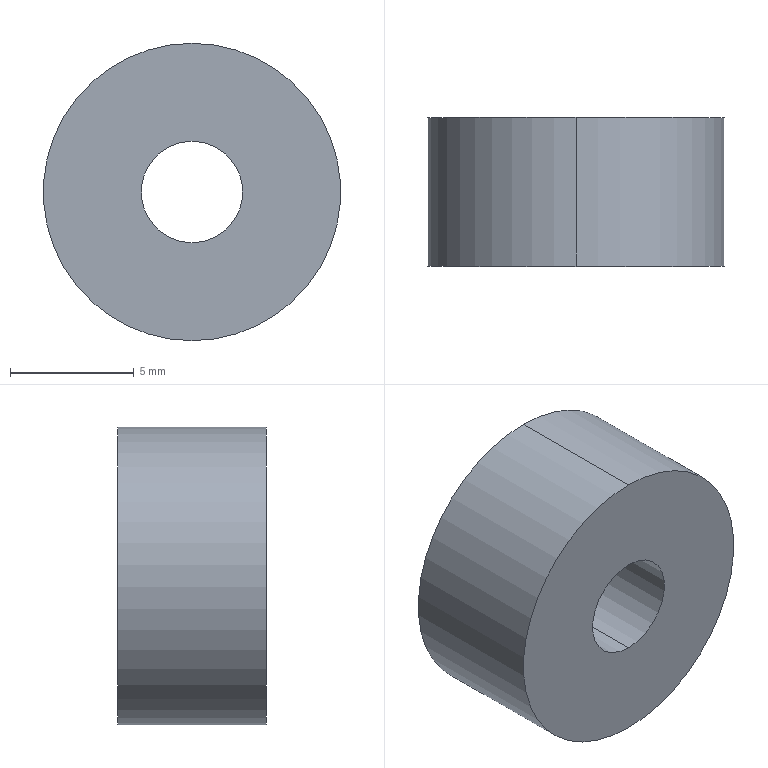Part | SolidWorks | features BaseBody 1 | 1 solid | 6 faces | box 12 x 6 x 12 mm | volume 599.369 mm3 | cylinder 4 | plane 2 | commonest cylinder face diameters 4.1 x2 12 x2
STEP:
#1=CARTESIAN_POINT('',(0.,3.,-6.));
#2=VERTEX_POINT('',#1);
#3=CARTESIAN_POINT('',(0.,3.,6.));
#4=VERTEX_POINT('',#3);
#5=CARTESIAN_POINT('',(0.,3.,0.));
#6=DIRECTION('',(0.,-1.,0.));
#7=DIRECTION('',(0.,0.,-1.));
#8=AXIS2_PLACEMENT_3D('',#5,#6,#7);
#9=CIRCLE('',#8,6.);
#10=EDGE_CURVE('',#2,#4,#9,.T.);
#11=ORIENTED_EDGE('',*,*,#10,.T.);
#12=CARTESIAN_POINT('',(0.,-3.,6.));
#13=VERTEX_POINT('',#12);
#14=CARTESIAN_POINT('',(0.,3.,6.));
#15=DIRECTION('',(0.,-1.,0.));
#16=VECTOR('',#15,1000.);
#17=LINE('',#14,#16);
#18=EDGE_CURVE('',#4,#13,#17,.T.);
#19=ORIENTED_EDGE('',*,*,#18,.T.);
#20=CARTESIAN_POINT('',(0.,-3.,-6.));
#21=VERTEX_POINT('',#20);
#22=CARTESIAN_POINT('',(0.,-3.,0.));
#23=DIRECTION('',(0.,1.,0.));
#24=DIRECTION('',(0.,0.,-1.));
#25=AXIS2_PLACEMENT_3D('',#22,#23,#24);
#26=CIRCLE('',#25,6.);
#27=EDGE_CURVE('',#13,#21,#26,.T.);
#28=ORIENTED_EDGE('',*,*,#27,.T.);
#29=CARTESIAN_POINT('',(0.,3.,-6.));
#30=DIRECTION('',(0.,-1.,0.));
#31=VECTOR('',#30,1000.);
#32=LINE('',#29,#31);
#33=EDGE_CURVE('',#2,#21,#32,.T.);
#34=ORIENTED_EDGE('',*,*,#33,.F.);
#35=EDGE_LOOP('',(#11,#19,#28,#34));
#36=FACE_OUTER_BOUND('',#35,.T.);
#37=CARTESIAN_POINT('',(0.,3.,0.));
#38=DIRECTION('',(0.,-1.,0.));
#39=DIRECTION('',(0.,0.,-1.));
#40=AXIS2_PLACEMENT_3D('',#37,#38,#39);
#41=CYLINDRICAL_SURFACE('',#40,6.);
#42=ADVANCED_FACE('',(#36),#41,.T.);
#43=CARTESIAN_POINT('',(0.,3.,2.05));
#44=VERTEX_POINT('',#43);
#45=CARTESIAN_POINT('',(0.,3.,-2.05));
#46=VERTEX_POINT('',#45);
#47=CARTESIAN_POINT('',(0.,3.,0.));
#48=DIRECTION('',(0.,-1.,0.));
#49=DIRECTION('',(0.,0.,-1.));
#50=AXIS2_PLACEMENT_3D('',#47,#48,#49);
#51=CIRCLE('',#50,2.05);
#52=EDGE_CURVE('',#44,#46,#51,.T.);
#53=ORIENTED_EDGE('',*,*,#52,.F.);
#54=CARTESIAN_POINT('',(0.,-3.,2.05));
#55=VERTEX_POINT('',#54);
#56=CARTESIAN_POINT('',(0.,3.,2.05));
#57=DIRECTION('',(0.,-1.,0.));
#58=VECTOR('',#57,1000.);
#59=LINE('',#56,#58);
#60=EDGE_CURVE('',#44,#55,#59,.T.);
#61=ORIENTED_EDGE('',*,*,#60,.T.);
#62=CARTESIAN_POINT('',(0.,-3.,-2.05));
#63=VERTEX_POINT('',#62);
#64=CARTESIAN_POINT('',(0.,-3.,0.));
#65=DIRECTION('',(0.,-1.,0.));
#66=DIRECTION('',(0.,0.,-1.));
#67=AXIS2_PLACEMENT_3D('',#64,#65,#66);
#68=CIRCLE('',#67,2.05);
#69=EDGE_CURVE('',#55,#63,#68,.T.);
#70=ORIENTED_EDGE('',*,*,#69,.T.);
#71=CARTESIAN_POINT('',(0.,3.,-2.05));
#72=DIRECTION('',(0.,-1.,0.));
#73=VECTOR('',#72,1000.);
#74=LINE('',#71,#73);
#75=EDGE_CURVE('',#46,#63,#74,.T.);
#76=ORIENTED_EDGE('',*,*,#75,.F.);
#77=EDGE_LOOP('',(#53,#61,#70,#76));
#78=FACE_OUTER_BOUND('',#77,.T.);
#79=CARTESIAN_POINT('',(0.,3.,0.));
#80=DIRECTION('',(0.,-1.,0.));
#81=DIRECTION('',(0.,0.,-1.));
#82=AXIS2_PLACEMENT_3D('',#79,#80,#81);
#83=CYLINDRICAL_SURFACE('',#82,2.05);
#84=ADVANCED_FACE('',(#78),#83,.F.);
#85=ORIENTED_EDGE('',*,*,#18,.F.);
#86=CARTESIAN_POINT('',(0.,3.,0.));
#87=DIRECTION('',(0.,-1.,0.));
#88=DIRECTION('',(0.,0.,-1.));
#89=AXIS2_PLACEMENT_3D('',#86,#87,#88);
#90=CIRCLE('',#89,6.);
#91=EDGE_CURVE('',#4,#2,#90,.T.);
#92=ORIENTED_EDGE('',*,*,#91,.T.);
#93=ORIENTED_EDGE('',*,*,#33,.T.);
#94=CARTESIAN_POINT('',(0.,-3.,0.));
#95=DIRECTION('',(0.,1.,0.));
#96=DIRECTION('',(0.,0.,-1.));
#97=AXIS2_PLACEMENT_3D('',#94,#95,#96);
#98=CIRCLE('',#97,6.);
#99=EDGE_CURVE('',#21,#13,#98,.T.);
#100=ORIENTED_EDGE('',*,*,#99,.T.);
#101=EDGE_LOOP('',(#85,#92,#93,#100));
#102=FACE_OUTER_BOUND('',#101,.T.);
#103=CARTESIAN_POINT('',(0.,3.,0.));
#104=DIRECTION('',(0.,-1.,0.));
#105=DIRECTION('',(0.,0.,-1.));
#106=AXIS2_PLACEMENT_3D('',#103,#104,#105);
#107=CYLINDRICAL_SURFACE('',#106,6.);
#108=ADVANCED_FACE('',(#102),#107,.T.);
#109=CARTESIAN_POINT('',(0.,-3.,0.));
#110=DIRECTION('',(0.,-1.,0.));
#111=DIRECTION('',(0.,0.,-1.));
#112=AXIS2_PLACEMENT_3D('',#109,#110,#111);
#113=CIRCLE('',#112,2.05);
#114=EDGE_CURVE('',#63,#55,#113,.T.);
#115=ORIENTED_EDGE('',*,*,#114,.F.);
#116=ORIENTED_EDGE('',*,*,#69,.F.);
#117=EDGE_LOOP('',(#115,#116));
#118=FACE_BOUND('',#117,.T.);
#119=ORIENTED_EDGE('',*,*,#99,.F.);
#120=ORIENTED_EDGE('',*,*,#27,.F.);
#121=EDGE_LOOP('',(#119,#120));
#122=FACE_OUTER_BOUND('',#121,.T.);
#123=CARTESIAN_POINT('',(0.,-3.,0.));
#124=DIRECTION('',(0.,1.,0.));
#125=DIRECTION('',(0.,0.,1.));
#126=AXIS2_PLACEMENT_3D('',#123,#124,#125);
#127=PLANE('',#126);
#128=ADVANCED_FACE('',(#118,#122),#127,.F.);
#129=CARTESIAN_POINT('',(0.,3.,0.));
#130=DIRECTION('',(0.,-1.,0.));
#131=DIRECTION('',(0.,0.,-1.));
#132=AXIS2_PLACEMENT_3D('',#129,#130,#131);
#133=CIRCLE('',#132,2.05);
#134=EDGE_CURVE('',#46,#44,#133,.T.);
#135=ORIENTED_EDGE('',*,*,#134,.T.);
#136=ORIENTED_EDGE('',*,*,#52,.T.);
#137=EDGE_LOOP('',(#135,#136));
#138=FACE_BOUND('',#137,.T.);
#139=ORIENTED_EDGE('',*,*,#10,.F.);
#140=ORIENTED_EDGE('',*,*,#91,.F.);
#141=EDGE_LOOP('',(#139,#140));
#142=FACE_OUTER_BOUND('',#141,.T.);
#143=CARTESIAN_POINT('',(0.,3.,0.));
#144=DIRECTION('',(0.,1.,0.));
#145=DIRECTION('',(0.,0.,1.));
#146=AXIS2_PLACEMENT_3D('',#143,#144,#145);
#147=PLANE('',#146);
#148=ADVANCED_FACE('',(#138,#142),#147,.T.);
#149=ORIENTED_EDGE('',*,*,#60,.F.);
#150=ORIENTED_EDGE('',*,*,#134,.F.);
#151=ORIENTED_EDGE('',*,*,#75,.T.);
#152=ORIENTED_EDGE('',*,*,#114,.T.);
#153=EDGE_LOOP('',(#149,#150,#151,#152));
#154=FACE_OUTER_BOUND('',#153,.T.);
#155=CARTESIAN_POINT('',(0.,3.,0.));
#156=DIRECTION('',(0.,-1.,0.));
#157=DIRECTION('',(0.,0.,-1.));
#158=AXIS2_PLACEMENT_3D('',#155,#156,#157);
#159=CYLINDRICAL_SURFACE('',#158,2.05);
#160=ADVANCED_FACE('',(#154),#159,.F.);
#161=CLOSED_SHELL('',(#42,#84,#108,#128,#148,#160));
#162=MANIFOLD_SOLID_BREP('',#161);
#163=CARTESIAN_POINT('',(0.,0.,0.));
#164=DIRECTION('',(0.,0.,1.));
#165=DIRECTION('',(1.,0.,0.));
#166=AXIS2_PLACEMENT_3D('',#163,#164,#165);
#167=(LENGTH_UNIT()NAMED_UNIT(*)SI_UNIT(.MILLI.,.METRE.));
#168=UNCERTAINTY_MEASURE_WITH_UNIT(LENGTH_MEASURE(0.00001),#167,'','');
#169=(NAMED_UNIT(*)PLANE_ANGLE_UNIT()SI_UNIT($,.RADIAN.));
#170=(NAMED_UNIT(*)SI_UNIT($,.STERADIAN.)SOLID_ANGLE_UNIT());
#171=(GEOMETRIC_REPRESENTATION_CONTEXT(3)GLOBAL_UNCERTAINTY_ASSIGNED_CONTEXT((#168))GLOBAL_UNIT_ASSIGNED_CONTEXT((#167,#169,#170))REPRESENTATION_CONTEXT('',''));
#172=ADVANCED_BREP_SHAPE_REPRESENTATION('',(#162,#166),#171);